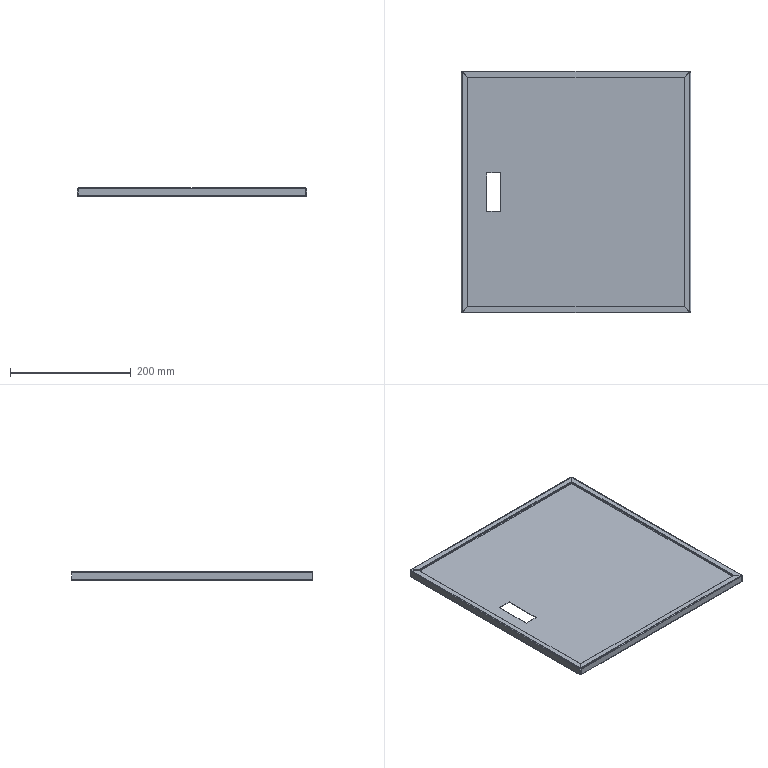Part | 1 solid | 74 faces | box 380 x 401 x 13.5 mm | volume 134987 mm3 | plane 42 | spline 16 | cylinder 16 | commonest cylinder face diameters 1.473 x8 2.946 x8